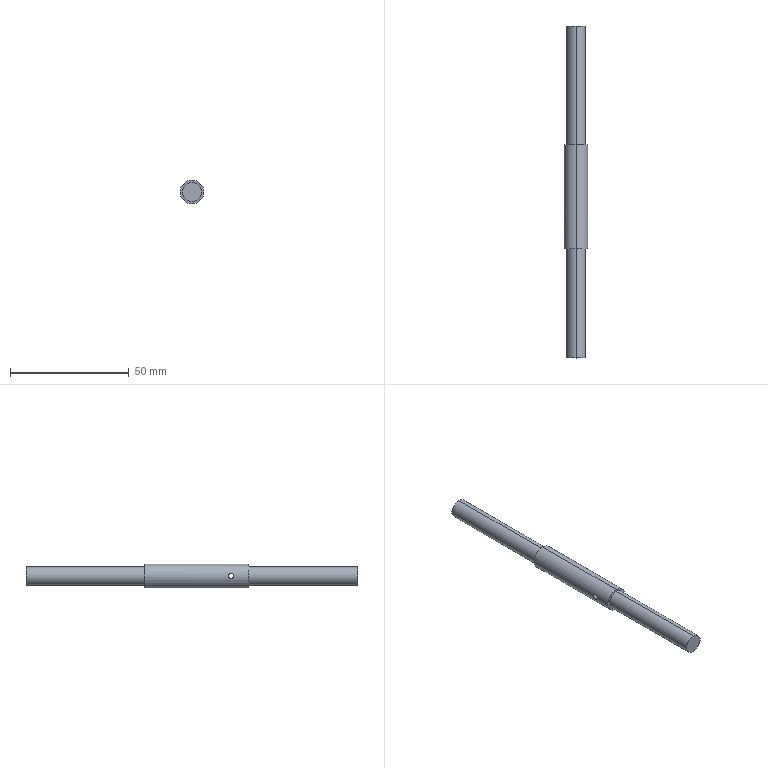Part | SolidWorks | features ICE 1, Revolution 1 | 1 solid | 12 faces | box 10 x 140 x 10 mm | volume 8243 mm3 | cylinder 8 | plane 4 | commonest cylinder face diameters 8 x4 2.2 x2 10 x2
STEP:
#1=CARTESIAN_POINT('',(-4.877,38.509,-1.1));
#2=VERTEX_POINT('',#1);
#3=CARTESIAN_POINT('',(-4.877,38.509,1.1));
#4=VERTEX_POINT('',#3);
#5=CARTESIAN_POINT('',(-4.877,38.509,-1.1));
#6=CARTESIAN_POINT('',(-4.877,38.363,-1.1));
#7=CARTESIAN_POINT('',(-4.884,38.22,-1.071));
#8=CARTESIAN_POINT('',(-4.907,37.954,-0.9605));
#9=CARTESIAN_POINT('',(-4.923,37.832,-0.8788));
#10=CARTESIAN_POINT('',(-4.955,37.63,-0.6765));
#11=CARTESIAN_POINT('',(-4.971,37.548,-0.5541));
#12=CARTESIAN_POINT('',(-4.993,37.438,-0.2895));
#13=CARTESIAN_POINT('',(-5.,37.409,-0.1444));
#14=CARTESIAN_POINT('',(-5.,37.409,0.1436));
#15=CARTESIAN_POINT('',(-4.993,37.437,0.2879));
#16=CARTESIAN_POINT('',(-4.971,37.548,0.5549));
#17=CARTESIAN_POINT('',(-4.955,37.629,0.6759));
#18=CARTESIAN_POINT('',(-4.923,37.833,0.8801));
#19=CARTESIAN_POINT('',(-4.907,37.955,0.9609));
#20=CARTESIAN_POINT('',(-4.884,38.22,1.071));
#21=CARTESIAN_POINT('',(-4.877,38.365,1.1));
#22=CARTESIAN_POINT('',(-4.877,38.509,1.1));
#23=B_SPLINE_CURVE_WITH_KNOTS('',3,(#5,#6,#7,#8,#9,#10,#11,#12,#13,#14,#15,#16,#17,#18,#19,#20,#21,#22),.UNSPECIFIED.,.F.,.F.,(4,2,2,2,2,2,2,2,4),(0.,0.0004312,0.0008624,0.001294,0.001725,0.002156,0.002587,0.003018,0.00345),.UNSPECIFIED.);
#24=EDGE_CURVE('',#2,#4,#23,.T.);
#25=ORIENTED_EDGE('',*,*,#24,.T.);
#26=CARTESIAN_POINT('',(4.877,38.509,1.1));
#27=VERTEX_POINT('',#26);
#28=CARTESIAN_POINT('',(-10.,38.509,1.1));
#29=DIRECTION('',(1.,0.,0.));
#30=VECTOR('',#29,1000.);
#31=LINE('',#28,#30);
#32=EDGE_CURVE('',#4,#27,#31,.T.);
#33=ORIENTED_EDGE('',*,*,#32,.T.);
#34=CARTESIAN_POINT('',(4.877,38.509,-1.1));
#35=VERTEX_POINT('',#34);
#36=CARTESIAN_POINT('',(4.877,38.509,1.1));
#37=CARTESIAN_POINT('',(4.877,38.365,1.1));
#38=CARTESIAN_POINT('',(4.884,38.22,1.071));
#39=CARTESIAN_POINT('',(4.907,37.955,0.9612));
#40=CARTESIAN_POINT('',(4.923,37.833,0.8796));
#41=CARTESIAN_POINT('',(4.955,37.63,0.6769));
#42=CARTESIAN_POINT('',(4.971,37.549,0.556));
#43=CARTESIAN_POINT('',(4.993,37.438,0.2888));
#44=CARTESIAN_POINT('',(5.,37.409,0.1457));
#45=CARTESIAN_POINT('',(5.,37.409,-0.1447));
#46=CARTESIAN_POINT('',(4.993,37.438,-0.2885));
#47=CARTESIAN_POINT('',(4.971,37.548,-0.5541));
#48=CARTESIAN_POINT('',(4.955,37.63,-0.6763));
#49=CARTESIAN_POINT('',(4.923,37.832,-0.8785));
#50=CARTESIAN_POINT('',(4.907,37.954,-0.9605));
#51=CARTESIAN_POINT('',(4.884,38.218,-1.071));
#52=CARTESIAN_POINT('',(4.877,38.363,-1.1));
#53=CARTESIAN_POINT('',(4.877,38.509,-1.1));
#54=B_SPLINE_CURVE_WITH_KNOTS('',3,(#36,#37,#38,#39,#40,#41,#42,#43,#44,#45,#46,#47,#48,#49,#50,#51,#52,#53),.UNSPECIFIED.,.F.,.F.,(4,2,2,2,2,2,2,2,4),(0.00345,0.003881,0.004312,0.004743,0.005174,0.005605,0.006036,0.006467,0.006898),.UNSPECIFIED.);
#55=EDGE_CURVE('',#27,#35,#54,.T.);
#56=ORIENTED_EDGE('',*,*,#55,.T.);
#57=CARTESIAN_POINT('',(-10.,38.509,-1.1));
#58=DIRECTION('',(1.,0.,0.));
#59=VECTOR('',#58,1000.);
#60=LINE('',#57,#59);
#61=EDGE_CURVE('',#2,#35,#60,.T.);
#62=ORIENTED_EDGE('',*,*,#61,.F.);
#63=EDGE_LOOP('',(#25,#33,#56,#62));
#64=FACE_OUTER_BOUND('',#63,.T.);
#65=CARTESIAN_POINT('',(-10.,38.509,0.));
#66=DIRECTION('',(1.,0.,0.));
#67=DIRECTION('',(0.,0.,-1.));
#68=AXIS2_PLACEMENT_3D('',#65,#66,#67);
#69=CYLINDRICAL_SURFACE('',#68,1.1);
#70=ADVANCED_FACE('',(#64),#69,.F.);
#71=CARTESIAN_POINT('',(0.,31.009,-4.));
#72=VERTEX_POINT('',#71);
#73=CARTESIAN_POINT('',(0.,31.009,4.));
#74=VERTEX_POINT('',#73);
#75=CARTESIAN_POINT('',(0.,31.009,0.));
#76=DIRECTION('',(0.,-1.,0.));
#77=DIRECTION('',(0.,0.,-1.));
#78=AXIS2_PLACEMENT_3D('',#75,#76,#77);
#79=CIRCLE('',#78,4.);
#80=EDGE_CURVE('',#72,#74,#79,.T.);
#81=ORIENTED_EDGE('',*,*,#80,.T.);
#82=CARTESIAN_POINT('',(0.,-14.991,4.));
#83=VERTEX_POINT('',#82);
#84=CARTESIAN_POINT('',(0.,0.,4.));
#85=DIRECTION('',(0.,-1.,0.));
#86=VECTOR('',#85,1000.);
#87=LINE('',#84,#86);
#88=EDGE_CURVE('',#74,#83,#87,.T.);
#89=ORIENTED_EDGE('',*,*,#88,.T.);
#90=CARTESIAN_POINT('',(0.,-14.991,-4.));
#91=VERTEX_POINT('',#90);
#92=CARTESIAN_POINT('',(0.,-14.991,0.));
#93=DIRECTION('',(0.,-1.,0.));
#94=DIRECTION('',(0.,0.,-1.));
#95=AXIS2_PLACEMENT_3D('',#92,#93,#94);
#96=CIRCLE('',#95,4.);
#97=EDGE_CURVE('',#91,#83,#96,.T.);
#98=ORIENTED_EDGE('',*,*,#97,.F.);
#99=CARTESIAN_POINT('',(0.,0.,-4.));
#100=DIRECTION('',(0.,-1.,0.));
#101=VECTOR('',#100,1000.);
#102=LINE('',#99,#101);
#103=EDGE_CURVE('',#72,#91,#102,.T.);
#104=ORIENTED_EDGE('',*,*,#103,.F.);
#105=EDGE_LOOP('',(#81,#89,#98,#104));
#106=FACE_OUTER_BOUND('',#105,.T.);
#107=CARTESIAN_POINT('',(0.,0.,0.));
#108=DIRECTION('',(0.,-1.,0.));
#109=DIRECTION('',(0.,0.,-1.));
#110=AXIS2_PLACEMENT_3D('',#107,#108,#109);
#111=CYLINDRICAL_SURFACE('',#110,4.);
#112=ADVANCED_FACE('',(#106),#111,.T.);
#113=CARTESIAN_POINT('',(4.877,38.509,-1.1));
#114=CARTESIAN_POINT('',(4.877,38.655,-1.1));
#115=CARTESIAN_POINT('',(4.884,38.798,-1.071));
#116=CARTESIAN_POINT('',(4.907,39.064,-0.9605));
#117=CARTESIAN_POINT('',(4.923,39.186,-0.8788));
#118=CARTESIAN_POINT('',(4.955,39.388,-0.6765));
#119=CARTESIAN_POINT('',(4.971,39.47,-0.5541));
#120=CARTESIAN_POINT('',(4.993,39.58,-0.2895));
#121=CARTESIAN_POINT('',(5.,39.609,-0.1444));
#122=CARTESIAN_POINT('',(5.,39.609,0.1436));
#123=CARTESIAN_POINT('',(4.993,39.58,0.2879));
#124=CARTESIAN_POINT('',(4.971,39.47,0.5549));
#125=CARTESIAN_POINT('',(4.955,39.389,0.6759));
#126=CARTESIAN_POINT('',(4.923,39.184,0.8801));
#127=CARTESIAN_POINT('',(4.907,39.063,0.9609));
#128=CARTESIAN_POINT('',(4.884,38.797,1.071));
#129=CARTESIAN_POINT('',(4.877,38.653,1.1));
#130=CARTESIAN_POINT('',(4.877,38.509,1.1));
#131=B_SPLINE_CURVE_WITH_KNOTS('',3,(#113,#114,#115,#116,#117,#118,#119,#120,#121,#122,#123,#124,#125,#126,#127,#128,#129,#130),.UNSPECIFIED.,.F.,.F.,(4,2,2,2,2,2,2,2,4),(0.,0.0004312,0.0008624,0.001294,0.001725,0.002156,0.002587,0.003018,0.00345),.UNSPECIFIED.);
#132=EDGE_CURVE('',#35,#27,#131,.T.);
#133=ORIENTED_EDGE('',*,*,#132,.F.);
#134=ORIENTED_EDGE('',*,*,#55,.F.);
#135=EDGE_LOOP('',(#133,#134));
#136=FACE_BOUND('',#135,.T.);
#137=CARTESIAN_POINT('',(0.,75.009,-5.));
#138=VERTEX_POINT('',#137);
#139=CARTESIAN_POINT('',(0.,75.009,5.));
#140=VERTEX_POINT('',#139);
#141=CARTESIAN_POINT('',(0.,75.009,0.));
#142=DIRECTION('',(0.,-1.,0.));
#143=DIRECTION('',(0.,0.,-1.));
#144=AXIS2_PLACEMENT_3D('',#141,#142,#143);
#145=CIRCLE('',#144,5.);
#146=EDGE_CURVE('',#138,#140,#145,.T.);
#147=ORIENTED_EDGE('',*,*,#146,.T.);
#148=CARTESIAN_POINT('',(0.,31.009,5.));
#149=VERTEX_POINT('',#148);
#150=CARTESIAN_POINT('',(0.,0.,5.));
#151=DIRECTION('',(0.,-1.,0.));
#152=VECTOR('',#151,1000.);
#153=LINE('',#150,#152);
#154=EDGE_CURVE('',#140,#149,#153,.T.);
#155=ORIENTED_EDGE('',*,*,#154,.T.);
#156=CARTESIAN_POINT('',(0.,31.009,-5.));
#157=VERTEX_POINT('',#156);
#158=CARTESIAN_POINT('',(0.,31.009,0.));
#159=DIRECTION('',(0.,-1.,0.));
#160=DIRECTION('',(0.,0.,-1.));
#161=AXIS2_PLACEMENT_3D('',#158,#159,#160);
#162=CIRCLE('',#161,5.);
#163=EDGE_CURVE('',#157,#149,#162,.T.);
#164=ORIENTED_EDGE('',*,*,#163,.F.);
#165=CARTESIAN_POINT('',(0.,0.,-5.));
#166=DIRECTION('',(0.,-1.,0.));
#167=VECTOR('',#166,1000.);
#168=LINE('',#165,#167);
#169=EDGE_CURVE('',#138,#157,#168,.T.);
#170=ORIENTED_EDGE('',*,*,#169,.F.);
#171=EDGE_LOOP('',(#147,#155,#164,#170));
#172=FACE_OUTER_BOUND('',#171,.T.);
#173=CARTESIAN_POINT('',(0.,0.,0.));
#174=DIRECTION('',(0.,-1.,0.));
#175=DIRECTION('',(0.,0.,-1.));
#176=AXIS2_PLACEMENT_3D('',#173,#174,#175);
#177=CYLINDRICAL_SURFACE('',#176,5.);
#178=ADVANCED_FACE('',(#136,#172),#177,.T.);
#179=CARTESIAN_POINT('',(0.,125.009,-4.));
#180=VERTEX_POINT('',#179);
#181=CARTESIAN_POINT('',(0.,125.009,4.));
#182=VERTEX_POINT('',#181);
#183=CARTESIAN_POINT('',(0.,125.009,0.));
#184=DIRECTION('',(0.,-1.,0.));
#185=DIRECTION('',(0.,0.,-1.));
#186=AXIS2_PLACEMENT_3D('',#183,#184,#185);
#187=CIRCLE('',#186,4.);
#188=EDGE_CURVE('',#180,#182,#187,.T.);
#189=ORIENTED_EDGE('',*,*,#188,.T.);
#190=CARTESIAN_POINT('',(0.,75.009,4.));
#191=VERTEX_POINT('',#190);
#192=CARTESIAN_POINT('',(0.,0.,4.));
#193=DIRECTION('',(0.,-1.,0.));
#194=VECTOR('',#193,1000.);
#195=LINE('',#192,#194);
#196=EDGE_CURVE('',#182,#191,#195,.T.);
#197=ORIENTED_EDGE('',*,*,#196,.T.);
#198=CARTESIAN_POINT('',(0.,75.009,-4.));
#199=VERTEX_POINT('',#198);
#200=CARTESIAN_POINT('',(0.,75.009,0.));
#201=DIRECTION('',(0.,-1.,0.));
#202=DIRECTION('',(0.,0.,-1.));
#203=AXIS2_PLACEMENT_3D('',#200,#201,#202);
#204=CIRCLE('',#203,4.);
#205=EDGE_CURVE('',#199,#191,#204,.T.);
#206=ORIENTED_EDGE('',*,*,#205,.F.);
#207=CARTESIAN_POINT('',(0.,0.,-4.));
#208=DIRECTION('',(0.,-1.,0.));
#209=VECTOR('',#208,1000.);
#210=LINE('',#207,#209);
#211=EDGE_CURVE('',#180,#199,#210,.T.);
#212=ORIENTED_EDGE('',*,*,#211,.F.);
#213=EDGE_LOOP('',(#189,#197,#206,#212));
#214=FACE_OUTER_BOUND('',#213,.T.);
#215=CARTESIAN_POINT('',(0.,0.,0.));
#216=DIRECTION('',(0.,-1.,0.));
#217=DIRECTION('',(0.,0.,-1.));
#218=AXIS2_PLACEMENT_3D('',#215,#216,#217);
#219=CYLINDRICAL_SURFACE('',#218,4.);
#220=ADVANCED_FACE('',(#214),#219,.T.);
#221=ORIENTED_EDGE('',*,*,#188,.F.);
#222=CARTESIAN_POINT('',(0.,125.009,0.));
#223=DIRECTION('',(0.,-1.,0.));
#224=DIRECTION('',(0.,0.,-1.));
#225=AXIS2_PLACEMENT_3D('',#222,#223,#224);
#226=CIRCLE('',#225,4.);
#227=EDGE_CURVE('',#182,#180,#226,.T.);
#228=ORIENTED_EDGE('',*,*,#227,.F.);
#229=EDGE_LOOP('',(#221,#228));
#230=FACE_OUTER_BOUND('',#229,.T.);
#231=CARTESIAN_POINT('',(0.,125.009,0.));
#232=DIRECTION('',(0.,1.,0.));
#233=DIRECTION('',(0.,0.,1.));
#234=AXIS2_PLACEMENT_3D('',#231,#232,#233);
#235=PLANE('',#234);
#236=ADVANCED_FACE('',(#230),#235,.T.);
#237=ORIENTED_EDGE('',*,*,#196,.F.);
#238=ORIENTED_EDGE('',*,*,#227,.T.);
#239=ORIENTED_EDGE('',*,*,#211,.T.);
#240=CARTESIAN_POINT('',(0.,75.009,0.));
#241=DIRECTION('',(0.,-1.,0.));
#242=DIRECTION('',(0.,0.,-1.));
#243=AXIS2_PLACEMENT_3D('',#240,#241,#242);
#244=CIRCLE('',#243,4.);
#245=EDGE_CURVE('',#191,#199,#244,.T.);
#246=ORIENTED_EDGE('',*,*,#245,.F.);
#247=EDGE_LOOP('',(#237,#238,#239,#246));
#248=FACE_OUTER_BOUND('',#247,.T.);
#249=CARTESIAN_POINT('',(0.,0.,0.));
#250=DIRECTION('',(0.,-1.,0.));
#251=DIRECTION('',(0.,0.,-1.));
#252=AXIS2_PLACEMENT_3D('',#249,#250,#251);
#253=CYLINDRICAL_SURFACE('',#252,4.);
#254=ADVANCED_FACE('',(#248),#253,.T.);
#255=ORIENTED_EDGE('',*,*,#205,.T.);
#256=ORIENTED_EDGE('',*,*,#245,.T.);
#257=EDGE_LOOP('',(#255,#256));
#258=FACE_BOUND('',#257,.T.);
#259=ORIENTED_EDGE('',*,*,#146,.F.);
#260=CARTESIAN_POINT('',(0.,75.009,0.));
#261=DIRECTION('',(0.,-1.,0.));
#262=DIRECTION('',(0.,0.,-1.));
#263=AXIS2_PLACEMENT_3D('',#260,#261,#262);
#264=CIRCLE('',#263,5.);
#265=EDGE_CURVE('',#140,#138,#264,.T.);
#266=ORIENTED_EDGE('',*,*,#265,.F.);
#267=EDGE_LOOP('',(#259,#266));
#268=FACE_OUTER_BOUND('',#267,.T.);
#269=CARTESIAN_POINT('',(4.,75.009,0.));
#270=DIRECTION('',(0.,1.,0.));
#271=DIRECTION('',(0.,0.,1.));
#272=AXIS2_PLACEMENT_3D('',#269,#270,#271);
#273=PLANE('',#272);
#274=ADVANCED_FACE('',(#258,#268),#273,.T.);
#275=ORIENTED_EDGE('',*,*,#154,.F.);
#276=ORIENTED_EDGE('',*,*,#265,.T.);
#277=ORIENTED_EDGE('',*,*,#169,.T.);
#278=CARTESIAN_POINT('',(0.,31.009,0.));
#279=DIRECTION('',(0.,-1.,0.));
#280=DIRECTION('',(0.,0.,-1.));
#281=AXIS2_PLACEMENT_3D('',#278,#279,#280);
#282=CIRCLE('',#281,5.);
#283=EDGE_CURVE('',#149,#157,#282,.T.);
#284=ORIENTED_EDGE('',*,*,#283,.F.);
#285=EDGE_LOOP('',(#275,#276,#277,#284));
#286=FACE_OUTER_BOUND('',#285,.T.);
#287=ORIENTED_EDGE('',*,*,#24,.F.);
#288=CARTESIAN_POINT('',(-4.877,38.509,1.1));
#289=CARTESIAN_POINT('',(-4.877,38.653,1.1));
#290=CARTESIAN_POINT('',(-4.884,38.798,1.071));
#291=CARTESIAN_POINT('',(-4.907,39.063,0.9612));
#292=CARTESIAN_POINT('',(-4.923,39.185,0.8796));
#293=CARTESIAN_POINT('',(-4.955,39.388,0.6769));
#294=CARTESIAN_POINT('',(-4.971,39.469,0.556));
#295=CARTESIAN_POINT('',(-4.993,39.58,0.2888));
#296=CARTESIAN_POINT('',(-5.,39.609,0.1457));
#297=CARTESIAN_POINT('',(-5.,39.609,-0.1447));
#298=CARTESIAN_POINT('',(-4.993,39.58,-0.2885));
#299=CARTESIAN_POINT('',(-4.971,39.47,-0.5541));
#300=CARTESIAN_POINT('',(-4.955,39.388,-0.6763));
#301=CARTESIAN_POINT('',(-4.923,39.186,-0.8785));
#302=CARTESIAN_POINT('',(-4.907,39.064,-0.9605));
#303=CARTESIAN_POINT('',(-4.884,38.799,-1.071));
#304=CARTESIAN_POINT('',(-4.877,38.655,-1.1));
#305=CARTESIAN_POINT('',(-4.877,38.509,-1.1));
#306=B_SPLINE_CURVE_WITH_KNOTS('',3,(#288,#289,#290,#291,#292,#293,#294,#295,#296,#297,#298,#299,#300,#301,#302,#303,#304,#305),.UNSPECIFIED.,.F.,.F.,(4,2,2,2,2,2,2,2,4),(0.00345,0.003881,0.004312,0.004743,0.005174,0.005605,0.006036,0.006467,0.006898),.UNSPECIFIED.);
#307=EDGE_CURVE('',#4,#2,#306,.T.);
#308=ORIENTED_EDGE('',*,*,#307,.F.);
#309=EDGE_LOOP('',(#287,#308));
#310=FACE_BOUND('',#309,.T.);
#311=CARTESIAN_POINT('',(0.,0.,0.));
#312=DIRECTION('',(0.,-1.,0.));
#313=DIRECTION('',(0.,0.,-1.));
#314=AXIS2_PLACEMENT_3D('',#311,#312,#313);
#315=CYLINDRICAL_SURFACE('',#314,5.);
#316=ADVANCED_FACE('',(#286,#310),#315,.T.);
#317=ORIENTED_EDGE('',*,*,#163,.T.);
#318=ORIENTED_EDGE('',*,*,#283,.T.);
#319=EDGE_LOOP('',(#317,#318));
#320=FACE_OUTER_BOUND('',#319,.T.);
#321=ORIENTED_EDGE('',*,*,#80,.F.);
#322=CARTESIAN_POINT('',(0.,31.009,0.));
#323=DIRECTION('',(0.,-1.,0.));
#324=DIRECTION('',(0.,0.,-1.));
#325=AXIS2_PLACEMENT_3D('',#322,#323,#324);
#326=CIRCLE('',#325,4.);
#327=EDGE_CURVE('',#74,#72,#326,.T.);
#328=ORIENTED_EDGE('',*,*,#327,.F.);
#329=EDGE_LOOP('',(#321,#328));
#330=FACE_BOUND('',#329,.T.);
#331=CARTESIAN_POINT('',(5.,31.009,0.));
#332=DIRECTION('',(0.,-1.,0.));
#333=DIRECTION('',(0.,0.,-1.));
#334=AXIS2_PLACEMENT_3D('',#331,#332,#333);
#335=PLANE('',#334);
#336=ADVANCED_FACE('',(#320,#330),#335,.T.);
#337=ORIENTED_EDGE('',*,*,#88,.F.);
#338=ORIENTED_EDGE('',*,*,#327,.T.);
#339=ORIENTED_EDGE('',*,*,#103,.T.);
#340=CARTESIAN_POINT('',(0.,-14.991,0.));
#341=DIRECTION('',(0.,-1.,0.));
#342=DIRECTION('',(0.,0.,-1.));
#343=AXIS2_PLACEMENT_3D('',#340,#341,#342);
#344=CIRCLE('',#343,4.);
#345=EDGE_CURVE('',#83,#91,#344,.T.);
#346=ORIENTED_EDGE('',*,*,#345,.F.);
#347=EDGE_LOOP('',(#337,#338,#339,#346));
#348=FACE_OUTER_BOUND('',#347,.T.);
#349=CARTESIAN_POINT('',(0.,0.,0.));
#350=DIRECTION('',(0.,-1.,0.));
#351=DIRECTION('',(0.,0.,-1.));
#352=AXIS2_PLACEMENT_3D('',#349,#350,#351);
#353=CYLINDRICAL_SURFACE('',#352,4.);
#354=ADVANCED_FACE('',(#348),#353,.T.);
#355=ORIENTED_EDGE('',*,*,#97,.T.);
#356=ORIENTED_EDGE('',*,*,#345,.T.);
#357=EDGE_LOOP('',(#355,#356));
#358=FACE_OUTER_BOUND('',#357,.T.);
#359=CARTESIAN_POINT('',(4.,-14.991,0.));
#360=DIRECTION('',(0.,-1.,0.));
#361=DIRECTION('',(0.,0.,-1.));
#362=AXIS2_PLACEMENT_3D('',#359,#360,#361);
#363=PLANE('',#362);
#364=ADVANCED_FACE('',(#358),#363,.T.);
#365=ORIENTED_EDGE('',*,*,#32,.F.);
#366=ORIENTED_EDGE('',*,*,#307,.T.);
#367=ORIENTED_EDGE('',*,*,#61,.T.);
#368=ORIENTED_EDGE('',*,*,#132,.T.);
#369=EDGE_LOOP('',(#365,#366,#367,#368));
#370=FACE_OUTER_BOUND('',#369,.T.);
#371=CARTESIAN_POINT('',(-10.,38.509,0.));
#372=DIRECTION('',(1.,0.,0.));
#373=DIRECTION('',(0.,0.,-1.));
#374=AXIS2_PLACEMENT_3D('',#371,#372,#373);
#375=CYLINDRICAL_SURFACE('',#374,1.1);
#376=ADVANCED_FACE('',(#370),#375,.F.);
#377=CLOSED_SHELL('',(#70,#112,#178,#220,#236,#254,#274,#316,#336,#354,#364,#376));
#378=MANIFOLD_SOLID_BREP('',#377);
#379=CARTESIAN_POINT('',(0.,0.,0.));
#380=DIRECTION('',(0.,0.,1.));
#381=DIRECTION('',(1.,0.,0.));
#382=AXIS2_PLACEMENT_3D('',#379,#380,#381);
#383=(LENGTH_UNIT()NAMED_UNIT(*)SI_UNIT(.MILLI.,.METRE.));
#384=UNCERTAINTY_MEASURE_WITH_UNIT(LENGTH_MEASURE(0.00001),#383,'','');
#385=(NAMED_UNIT(*)PLANE_ANGLE_UNIT()SI_UNIT($,.RADIAN.));
#386=(NAMED_UNIT(*)SI_UNIT($,.STERADIAN.)SOLID_ANGLE_UNIT());
#387=(GEOMETRIC_REPRESENTATION_CONTEXT(3)GLOBAL_UNCERTAINTY_ASSIGNED_CONTEXT((#384))GLOBAL_UNIT_ASSIGNED_CONTEXT((#383,#385,#386))REPRESENTATION_CONTEXT('',''));
#388=ADVANCED_BREP_SHAPE_REPRESENTATION('',(#378,#382),#387);